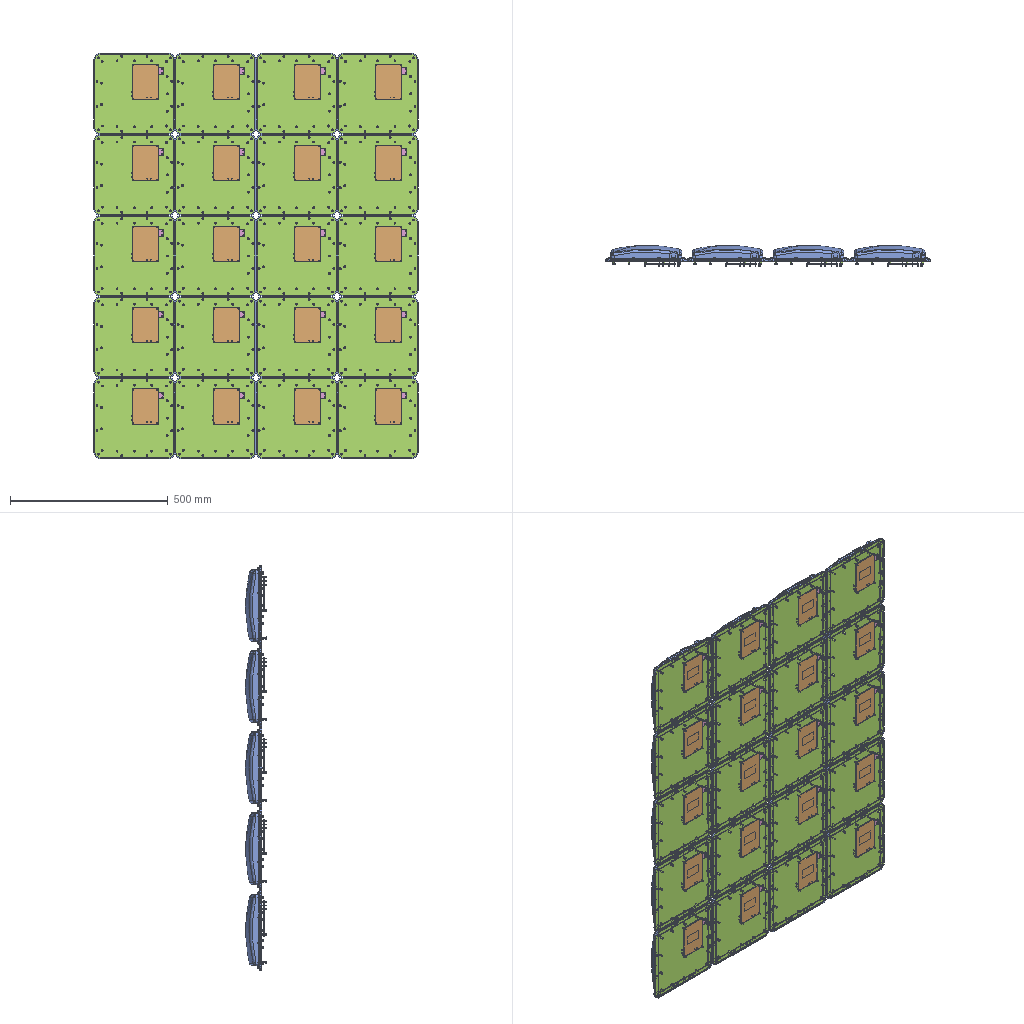Assembly | SolidWorks | 6 different items | 120 placed | box 1028 x 67 x 1285 mm
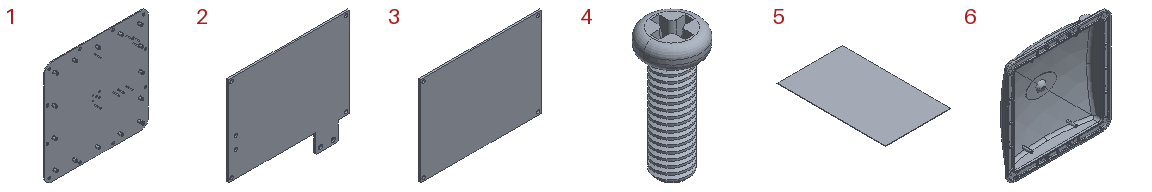Parts list (item | quantity | size | volume | features):
1 | x20 | 250.5 x 17 x 250.5 mm | 127405 mm3 | features Chamfer 2, ICE 2, Cut 1, Extrusion 1, HoleWzd 1
2 | x20 | 111.5 x 1.7 x 100.35 mm | 16166 mm3 | features Extrusion 1
3 | x20 | 111.5 x 1.75 x 82.6 mm | 16068 mm3 | features Extrusion 1
4 | x20 | 6.5 x 6.5 x 14.5 mm | 192.159 mm3 | features Fillet 2, ICE 2, Chamfer 1, Extrusion 1, Helix 1, SweepCut 1
5 | x20 | 30 x 50 x 0.2 mm | 300 mm3 | features Extrusion 1
6 | x20 | 257 x 51.2 x 257 mm | 287758 mm3 | features ICE 12, Fillet 3, Revolution 3, MirrorPattern 2, RevCut 2, 3DProfileFeature 1, CirPattern 1, Extrusion 1, HoleWzd 1, Rib 1, Shell 1, SweepCut 1
Mates (type | each side: item.copy, entity, surface, feature):
Coordinate | 6.1 select_type:25 | assembly select_type:11
Coincident | 1.1 plane | assembly plane | 2 times
Coincident | 6.1 face plane Cut-Extrude 1 | 1.1 face plane Boss-Extrude 1
Parallel | 2.1 plane | assembly plane | 2 times
InPlace | 2.1 face plane Boss-Extrude 1 | 5.1 plane
Coincident | 5.1 face plane Boss-Extrude 1 | 3.1 face plane Boss-Extrude 1
Concentric | 1.1 edge | 3.1 face cylinder Boss-Extrude 1
Parallel | 2.1 face plane Boss-Extrude 1 | 3.1 face plane Boss-Extrude 1
Concentric | 1.1 edge | 4.1 edge
DistanceDim | 4.1 face plane Boss-Extrude 2 | 1.1 face plane Boss-Extrude 2